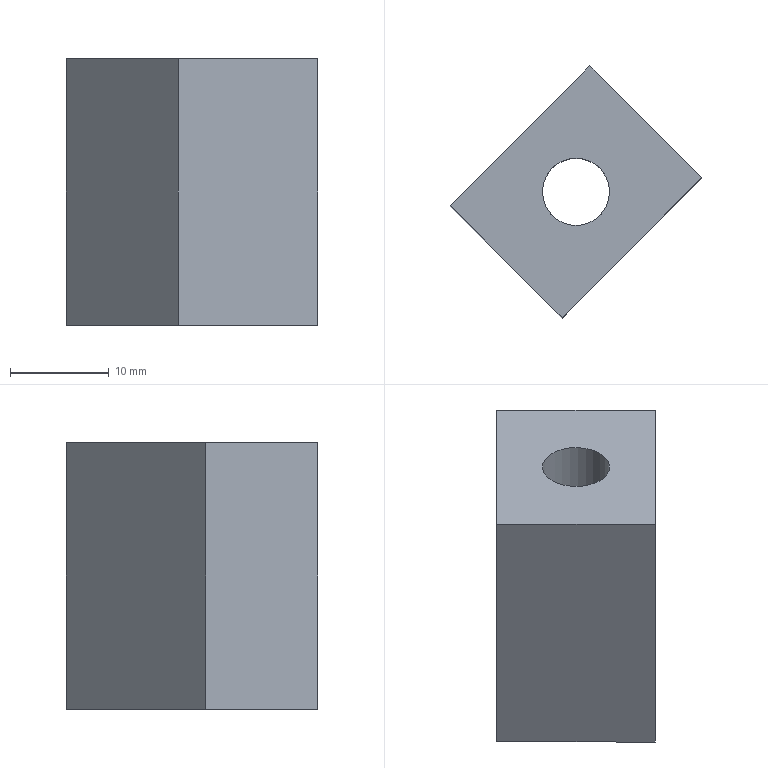Part | STEP file | gslz 2016.10.28-13_id1478_x_t | 1 solid | 9 faces | box 25.456 x 25.456 x 27 mm | volume 6738 mm3 | plane 7 | cylinder 2 | commonest cylinder face diameters 6.8 x1 12 x1
STEP:
#1=CARTESIAN_POINT('',(0.,0.,0.));
#2=DIRECTION('',(0.,0.,1.));
#3=DIRECTION('',(1.,0.,0.));
#4=AXIS2_PLACEMENT_3D('',#1,#2,#3);
#5=CARTESIAN_POINT('',(612.273,213.143,-70.5));
#6=VERTEX_POINT('',#5);
#7=CARTESIAN_POINT('',(608.873,213.143,-70.5));
#8=DIRECTION('',(0.,0.,-1.));
#9=DIRECTION('',(1.,0.,0.));
#10=AXIS2_PLACEMENT_3D('',#7,#8,#9);
#11=CIRCLE('',#10,3.4);
#12=CARTESIAN_POINT('',(628.559,232.788,-70.5));
#13=DIRECTION('',(0.,0.,1.));
#14=DIRECTION('',(1.,0.,0.));
#15=AXIS2_PLACEMENT_3D('',#12,#13,#14);
#16=PLANE('',#15);
#17=CARTESIAN_POINT('',(-16.286,-19.645));
#18=CARTESIAN_POINT('',(-16.286,-25.534));
#19=CARTESIAN_POINT('',(-21.386,-22.59));
#20=CARTESIAN_POINT('',(-26.486,-19.645));
#21=CARTESIAN_POINT('',(-21.386,-16.701));
#22=CARTESIAN_POINT('',(-16.286,-13.756));
#23=CARTESIAN_POINT('',(-16.286,-19.645));
#24=(BOUNDED_CURVE()B_SPLINE_CURVE(2,(#17,#18,#19,#20,#21,#22,#23),.UNSPECIFIED.,.T.,.F.)B_SPLINE_CURVE_WITH_KNOTS((1,2,2,2,2,1),(-2.094,0.,2.094,4.189,6.283,8.378),.UNSPECIFIED.)CURVE()GEOMETRIC_REPRESENTATION_ITEM()RATIONAL_B_SPLINE_CURVE((1.,0.5,1.,0.5,1.,0.5,1.))REPRESENTATION_ITEM(''));
#25=(GEOMETRIC_REPRESENTATION_CONTEXT(2)PARAMETRIC_REPRESENTATION_CONTEXT()REPRESENTATION_CONTEXT('',''));
#26=DEFINITIONAL_REPRESENTATION('',(#24),#25);
#27=PCURVE('',#16,#26);
#28=CARTESIAN_POINT('',(608.873,213.143,-55.5));
#29=DIRECTION('',(0.,0.,1.));
#30=DIRECTION('',(1.,0.,0.));
#31=AXIS2_PLACEMENT_3D('',#28,#29,#30);
#32=CYLINDRICAL_SURFACE('',#31,3.4);
#33=CARTESIAN_POINT('',(6.283,-15.));
#34=DIRECTION('',(-1.,0.));
#35=VECTOR('',#34,1.);
#36=LINE('',#33,#35);
#37=(GEOMETRIC_REPRESENTATION_CONTEXT(2)PARAMETRIC_REPRESENTATION_CONTEXT()REPRESENTATION_CONTEXT('',''));
#38=DEFINITIONAL_REPRESENTATION('',(#36),#37);
#39=PCURVE('',#32,#38);
#40=SURFACE_CURVE('',#11,(#27,#39),.PCURVE_S1.);
#41=EDGE_CURVE('',#6,#6,#40,.T.);
#42=ORIENTED_EDGE('',*,*,#41,.T.);
#43=EDGE_LOOP('',(#42));
#44=FACE_BOUND('',#43,.T.);
#45=CARTESIAN_POINT('',(621.601,214.557,-70.5));
#46=VERTEX_POINT('',#45);
#47=CARTESIAN_POINT('',(607.459,200.415,-70.5));
#48=VERTEX_POINT('',#47);
#49=CARTESIAN_POINT('',(623.015,215.971,-70.5));
#50=DIRECTION('',(-0.7071,-0.7071,0.));
#51=VECTOR('',#50,1.);
#52=LINE('',#49,#51);
#53=CARTESIAN_POINT('',(-5.544,-16.817));
#54=DIRECTION('',(-0.7071,-0.7071));
#55=VECTOR('',#54,1.);
#56=LINE('',#53,#55);
#57=(GEOMETRIC_REPRESENTATION_CONTEXT(2)PARAMETRIC_REPRESENTATION_CONTEXT()REPRESENTATION_CONTEXT('',''));
#58=DEFINITIONAL_REPRESENTATION('',(#56),#57);
#59=PCURVE('',#16,#58);
#60=CARTESIAN_POINT('',(623.015,215.971,-93.));
#61=DIRECTION('',(-0.7071,0.7071,0.));
#62=DIRECTION('',(-0.7071,-0.7071,0.));
#63=AXIS2_PLACEMENT_3D('',#60,#61,#62);
#64=PLANE('',#63);
#65=CARTESIAN_POINT('',(0.,22.5));
#66=DIRECTION('',(1.,0.));
#67=VECTOR('',#66,1.);
#68=LINE('',#65,#67);
#69=(GEOMETRIC_REPRESENTATION_CONTEXT(2)PARAMETRIC_REPRESENTATION_CONTEXT()REPRESENTATION_CONTEXT('',''));
#70=DEFINITIONAL_REPRESENTATION('',(#68),#69);
#71=PCURVE('',#64,#70);
#72=SURFACE_CURVE('',#52,(#59,#71),.PCURVE_S1.);
#73=EDGE_CURVE('',#46,#48,#72,.T.);
#74=ORIENTED_EDGE('',*,*,#73,.F.);
#75=CARTESIAN_POINT('',(610.287,225.87,-70.5));
#76=VERTEX_POINT('',#75);
#77=CARTESIAN_POINT('',(615.944,220.214,-70.5));
#78=DIRECTION('',(0.7071,-0.7071,0.));
#79=VECTOR('',#78,1.);
#80=LINE('',#77,#79);
#81=CARTESIAN_POINT('',(-12.615,-12.574));
#82=DIRECTION('',(0.7071,-0.7071));
#83=VECTOR('',#82,1.);
#84=LINE('',#81,#83);
#85=(GEOMETRIC_REPRESENTATION_CONTEXT(2)PARAMETRIC_REPRESENTATION_CONTEXT()REPRESENTATION_CONTEXT('',''));
#86=DEFINITIONAL_REPRESENTATION('',(#84),#85);
#87=PCURVE('',#16,#86);
#88=CARTESIAN_POINT('',(615.944,220.214,-93.));
#89=DIRECTION('',(-0.7071,-0.7071,0.));
#90=DIRECTION('',(0.7071,-0.7071,0.));
#91=AXIS2_PLACEMENT_3D('',#88,#89,#90);
#92=PLANE('',#91);
#93=CARTESIAN_POINT('',(0.,22.5));
#94=DIRECTION('',(1.,0.));
#95=VECTOR('',#94,1.);
#96=LINE('',#93,#95);
#97=(GEOMETRIC_REPRESENTATION_CONTEXT(2)PARAMETRIC_REPRESENTATION_CONTEXT()REPRESENTATION_CONTEXT('',''));
#98=DEFINITIONAL_REPRESENTATION('',(#96),#97);
#99=PCURVE('',#92,#98);
#100=SURFACE_CURVE('',#80,(#87,#99),.PCURVE_S1.);
#101=EDGE_CURVE('',#76,#46,#100,.T.);
#102=ORIENTED_EDGE('',*,*,#101,.F.);
#103=CARTESIAN_POINT('',(596.145,211.728,-70.5));
#104=VERTEX_POINT('',#103);
#105=CARTESIAN_POINT('',(611.701,227.285,-70.5));
#106=DIRECTION('',(-0.7071,-0.7071,0.));
#107=VECTOR('',#106,1.);
#108=LINE('',#105,#107);
#109=CARTESIAN_POINT('',(-16.858,-5.503));
#110=DIRECTION('',(-0.7071,-0.7071));
#111=VECTOR('',#110,1.);
#112=LINE('',#109,#111);
#113=(GEOMETRIC_REPRESENTATION_CONTEXT(2)PARAMETRIC_REPRESENTATION_CONTEXT()REPRESENTATION_CONTEXT('',''));
#114=DEFINITIONAL_REPRESENTATION('',(#112),#113);
#115=PCURVE('',#16,#114);
#116=CARTESIAN_POINT('',(611.701,227.285,-93.));
#117=DIRECTION('',(-0.7071,0.7071,0.));
#118=DIRECTION('',(-0.7071,-0.7071,0.));
#119=AXIS2_PLACEMENT_3D('',#116,#117,#118);
#120=PLANE('',#119);
#121=CARTESIAN_POINT('',(0.,22.5));
#122=DIRECTION('',(1.,0.));
#123=VECTOR('',#122,1.);
#124=LINE('',#121,#123);
#125=(GEOMETRIC_REPRESENTATION_CONTEXT(2)PARAMETRIC_REPRESENTATION_CONTEXT()REPRESENTATION_CONTEXT('',''));
#126=DEFINITIONAL_REPRESENTATION('',(#124),#125);
#127=PCURVE('',#120,#126);
#128=SURFACE_CURVE('',#108,(#115,#127),.PCURVE_S1.);
#129=EDGE_CURVE('',#76,#104,#128,.T.);
#130=ORIENTED_EDGE('',*,*,#129,.T.);
#131=CARTESIAN_POINT('',(601.822,206.051,-70.5));
#132=DIRECTION('',(0.7071,-0.7071,0.));
#133=VECTOR('',#132,1.);
#134=LINE('',#131,#133);
#135=CARTESIAN_POINT('',(-26.737,-26.737));
#136=DIRECTION('',(0.7071,-0.7071));
#137=VECTOR('',#136,1.);
#138=LINE('',#135,#137);
#139=(GEOMETRIC_REPRESENTATION_CONTEXT(2)PARAMETRIC_REPRESENTATION_CONTEXT()REPRESENTATION_CONTEXT('',''));
#140=DEFINITIONAL_REPRESENTATION('',(#138),#139);
#141=PCURVE('',#16,#140);
#142=CARTESIAN_POINT('',(601.822,206.051,-58.639));
#143=DIRECTION('',(0.7071,0.7071,0.));
#144=DIRECTION('',(-0.7071,0.7071,0.));
#145=AXIS2_PLACEMENT_3D('',#142,#143,#144);
#146=PLANE('',#145);
#147=CARTESIAN_POINT('',(0.,-11.861));
#148=DIRECTION('',(-1.,0.));
#149=VECTOR('',#148,1.);
#150=LINE('',#147,#149);
#151=(GEOMETRIC_REPRESENTATION_CONTEXT(2)PARAMETRIC_REPRESENTATION_CONTEXT()REPRESENTATION_CONTEXT('',''));
#152=DEFINITIONAL_REPRESENTATION('',(#150),#151);
#153=PCURVE('',#146,#152);
#154=SURFACE_CURVE('',#134,(#141,#153),.PCURVE_S1.);
#155=EDGE_CURVE('',#104,#48,#154,.T.);
#156=ORIENTED_EDGE('',*,*,#155,.T.);
#157=EDGE_LOOP('',(#74,#102,#130,#156));
#158=FACE_BOUND('',#157,.T.);
#159=ADVANCED_FACE('',(#44,#158),#16,.T.);
#160=CARTESIAN_POINT('',(621.601,214.557,-97.5));
#161=VERTEX_POINT('',#160);
#162=CARTESIAN_POINT('',(607.459,200.415,-97.5));
#163=VERTEX_POINT('',#162);
#164=CARTESIAN_POINT('',(623.015,215.971,-97.5));
#165=DIRECTION('',(-0.7071,-0.7071,0.));
#166=VECTOR('',#165,1.);
#167=LINE('',#164,#166);
#168=CARTESIAN_POINT('',(0.,-4.5));
#169=DIRECTION('',(1.,0.));
#170=VECTOR('',#169,1.);
#171=LINE('',#168,#170);
#172=(GEOMETRIC_REPRESENTATION_CONTEXT(2)PARAMETRIC_REPRESENTATION_CONTEXT()REPRESENTATION_CONTEXT('',''));
#173=DEFINITIONAL_REPRESENTATION('',(#171),#172);
#174=PCURVE('',#64,#173);
#175=CARTESIAN_POINT('',(617.358,221.628,-97.5));
#176=DIRECTION('',(0.,0.,1.));
#177=DIRECTION('',(1.,0.,0.));
#178=AXIS2_PLACEMENT_3D('',#175,#176,#177);
#179=PLANE('',#178);
#180=CARTESIAN_POINT('',(5.657,-5.657));
#181=DIRECTION('',(-0.7071,-0.7071));
#182=VECTOR('',#181,1.);
#183=LINE('',#180,#182);
#184=(GEOMETRIC_REPRESENTATION_CONTEXT(2)PARAMETRIC_REPRESENTATION_CONTEXT()REPRESENTATION_CONTEXT('',''));
#185=DEFINITIONAL_REPRESENTATION('',(#183),#184);
#186=PCURVE('',#179,#185);
#187=SURFACE_CURVE('',#167,(#174,#186),.PCURVE_S1.);
#188=EDGE_CURVE('',#161,#163,#187,.T.);
#189=ORIENTED_EDGE('',*,*,#188,.F.);
#190=CARTESIAN_POINT('',(621.601,214.557,-93.));
#191=DIRECTION('',(0.,0.,1.));
#192=VECTOR('',#191,1.);
#193=LINE('',#190,#192);
#194=CARTESIAN_POINT('',(2.,0.));
#195=DIRECTION('',(0.,1.));
#196=VECTOR('',#195,1.);
#197=LINE('',#194,#196);
#198=(GEOMETRIC_REPRESENTATION_CONTEXT(2)PARAMETRIC_REPRESENTATION_CONTEXT()REPRESENTATION_CONTEXT('',''));
#199=DEFINITIONAL_REPRESENTATION('',(#197),#198);
#200=PCURVE('',#64,#199);
#201=CARTESIAN_POINT('',(8.,0.));
#202=DIRECTION('',(0.,1.));
#203=VECTOR('',#202,1.);
#204=LINE('',#201,#203);
#205=(GEOMETRIC_REPRESENTATION_CONTEXT(2)PARAMETRIC_REPRESENTATION_CONTEXT()REPRESENTATION_CONTEXT('',''));
#206=DEFINITIONAL_REPRESENTATION('',(#204),#205);
#207=PCURVE('',#92,#206);
#208=SURFACE_CURVE('',#193,(#200,#207),.PCURVE_S1.);
#209=EDGE_CURVE('',#161,#46,#208,.T.);
#210=ORIENTED_EDGE('',*,*,#209,.T.);
#211=ORIENTED_EDGE('',*,*,#73,.T.);
#212=CARTESIAN_POINT('',(607.459,200.415,-93.));
#213=DIRECTION('',(0.,0.,1.));
#214=VECTOR('',#213,1.);
#215=LINE('',#212,#214);
#216=CARTESIAN_POINT('',(22.,0.));
#217=DIRECTION('',(0.,1.));
#218=VECTOR('',#217,1.);
#219=LINE('',#216,#218);
#220=(GEOMETRIC_REPRESENTATION_CONTEXT(2)PARAMETRIC_REPRESENTATION_CONTEXT()REPRESENTATION_CONTEXT('',''));
#221=DEFINITIONAL_REPRESENTATION('',(#219),#220);
#222=PCURVE('',#64,#221);
#223=CARTESIAN_POINT('',(-7.971,-34.361));
#224=DIRECTION('',(0.,1.));
#225=VECTOR('',#224,1.);
#226=LINE('',#223,#225);
#227=(GEOMETRIC_REPRESENTATION_CONTEXT(2)PARAMETRIC_REPRESENTATION_CONTEXT()REPRESENTATION_CONTEXT('',''));
#228=DEFINITIONAL_REPRESENTATION('',(#226),#227);
#229=PCURVE('',#146,#228);
#230=SURFACE_CURVE('',#215,(#222,#229),.PCURVE_S1.);
#231=EDGE_CURVE('',#163,#48,#230,.T.);
#232=ORIENTED_EDGE('',*,*,#231,.F.);
#233=EDGE_LOOP('',(#189,#210,#211,#232));
#234=FACE_BOUND('',#233,.T.);
#235=ADVANCED_FACE('',(#234),#64,.F.);
#236=CARTESIAN_POINT('',(614.873,213.143,-97.5));
#237=VERTEX_POINT('',#236);
#238=CARTESIAN_POINT('',(608.873,213.143,-97.5));
#239=DIRECTION('',(0.,0.,1.));
#240=DIRECTION('',(1.,0.,0.));
#241=AXIS2_PLACEMENT_3D('',#238,#239,#240);
#242=CIRCLE('',#241,6.);
#243=CARTESIAN_POINT('',(-8.485,-8.485));
#244=DIRECTION('',(1.,0.));
#245=AXIS2_PLACEMENT_2D('',#243,#244);
#246=CIRCLE('',#245,6.);
#247=(GEOMETRIC_REPRESENTATION_CONTEXT(2)PARAMETRIC_REPRESENTATION_CONTEXT()REPRESENTATION_CONTEXT('',''));
#248=DEFINITIONAL_REPRESENTATION('',(#246),#247);
#249=PCURVE('',#179,#248);
#250=CARTESIAN_POINT('',(608.873,213.143,-105.5));
#251=DIRECTION('',(0.,0.,1.));
#252=DIRECTION('',(1.,0.,0.));
#253=AXIS2_PLACEMENT_3D('',#250,#251,#252);
#254=CYLINDRICAL_SURFACE('',#253,6.);
#255=CARTESIAN_POINT('',(0.,8.));
#256=DIRECTION('',(1.,0.));
#257=VECTOR('',#256,1.);
#258=LINE('',#255,#257);
#259=(GEOMETRIC_REPRESENTATION_CONTEXT(2)PARAMETRIC_REPRESENTATION_CONTEXT()REPRESENTATION_CONTEXT('',''));
#260=DEFINITIONAL_REPRESENTATION('',(#258),#259);
#261=PCURVE('',#254,#260);
#262=SURFACE_CURVE('',#242,(#249,#261),.PCURVE_S1.);
#263=EDGE_CURVE('',#237,#237,#262,.T.);
#264=ORIENTED_EDGE('',*,*,#263,.T.);
#265=EDGE_LOOP('',(#264));
#266=FACE_BOUND('',#265,.T.);
#267=CARTESIAN_POINT('',(610.287,225.87,-97.5));
#268=VERTEX_POINT('',#267);
#269=CARTESIAN_POINT('',(615.944,220.214,-97.5));
#270=DIRECTION('',(-0.7071,0.7071,0.));
#271=VECTOR('',#270,1.);
#272=LINE('',#269,#271);
#273=CARTESIAN_POINT('',(-1.414,-1.414));
#274=DIRECTION('',(-0.7071,0.7071));
#275=VECTOR('',#274,1.);
#276=LINE('',#273,#275);
#277=(GEOMETRIC_REPRESENTATION_CONTEXT(2)PARAMETRIC_REPRESENTATION_CONTEXT()REPRESENTATION_CONTEXT('',''));
#278=DEFINITIONAL_REPRESENTATION('',(#276),#277);
#279=PCURVE('',#179,#278);
#280=CARTESIAN_POINT('',(0.,-4.5));
#281=DIRECTION('',(-1.,0.));
#282=VECTOR('',#281,1.);
#283=LINE('',#280,#282);
#284=(GEOMETRIC_REPRESENTATION_CONTEXT(2)PARAMETRIC_REPRESENTATION_CONTEXT()REPRESENTATION_CONTEXT('',''));
#285=DEFINITIONAL_REPRESENTATION('',(#283),#284);
#286=PCURVE('',#92,#285);
#287=SURFACE_CURVE('',#272,(#279,#286),.PCURVE_S1.);
#288=EDGE_CURVE('',#161,#268,#287,.T.);
#289=ORIENTED_EDGE('',*,*,#288,.F.);
#290=ORIENTED_EDGE('',*,*,#188,.T.);
#291=CARTESIAN_POINT('',(596.145,211.728,-97.5));
#292=VERTEX_POINT('',#291);
#293=CARTESIAN_POINT('',(601.822,206.051,-97.5));
#294=DIRECTION('',(-0.7071,0.7071,0.));
#295=VECTOR('',#294,1.);
#296=LINE('',#293,#295);
#297=CARTESIAN_POINT('',(-15.536,-15.577));
#298=DIRECTION('',(-0.7071,0.7071));
#299=VECTOR('',#298,1.);
#300=LINE('',#297,#299);
#301=(GEOMETRIC_REPRESENTATION_CONTEXT(2)PARAMETRIC_REPRESENTATION_CONTEXT()REPRESENTATION_CONTEXT('',''));
#302=DEFINITIONAL_REPRESENTATION('',(#300),#301);
#303=PCURVE('',#179,#302);
#304=CARTESIAN_POINT('',(0.,-38.861));
#305=DIRECTION('',(1.,0.));
#306=VECTOR('',#305,1.);
#307=LINE('',#304,#306);
#308=(GEOMETRIC_REPRESENTATION_CONTEXT(2)PARAMETRIC_REPRESENTATION_CONTEXT()REPRESENTATION_CONTEXT('',''));
#309=DEFINITIONAL_REPRESENTATION('',(#307),#308);
#310=PCURVE('',#146,#309);
#311=SURFACE_CURVE('',#296,(#303,#310),.PCURVE_S1.);
#312=EDGE_CURVE('',#163,#292,#311,.T.);
#313=ORIENTED_EDGE('',*,*,#312,.T.);
#314=CARTESIAN_POINT('',(611.701,227.285,-97.5));
#315=DIRECTION('',(-0.7071,-0.7071,0.));
#316=VECTOR('',#315,1.);
#317=LINE('',#314,#316);
#318=CARTESIAN_POINT('',(-5.657,5.657));
#319=DIRECTION('',(-0.7071,-0.7071));
#320=VECTOR('',#319,1.);
#321=LINE('',#318,#320);
#322=(GEOMETRIC_REPRESENTATION_CONTEXT(2)PARAMETRIC_REPRESENTATION_CONTEXT()REPRESENTATION_CONTEXT('',''));
#323=DEFINITIONAL_REPRESENTATION('',(#321),#322);
#324=PCURVE('',#179,#323);
#325=CARTESIAN_POINT('',(0.,-4.5));
#326=DIRECTION('',(1.,0.));
#327=VECTOR('',#326,1.);
#328=LINE('',#325,#327);
#329=(GEOMETRIC_REPRESENTATION_CONTEXT(2)PARAMETRIC_REPRESENTATION_CONTEXT()REPRESENTATION_CONTEXT('',''));
#330=DEFINITIONAL_REPRESENTATION('',(#328),#329);
#331=PCURVE('',#120,#330);
#332=SURFACE_CURVE('',#317,(#324,#331),.PCURVE_S1.);
#333=EDGE_CURVE('',#268,#292,#332,.T.);
#334=ORIENTED_EDGE('',*,*,#333,.F.);
#335=EDGE_LOOP('',(#289,#290,#313,#334));
#336=FACE_BOUND('',#335,.T.);
#337=ADVANCED_FACE('',(#266,#336),#179,.F.);
#338=ORIENTED_EDGE('',*,*,#129,.F.);
#339=CARTESIAN_POINT('',(610.287,225.87,-93.));
#340=DIRECTION('',(0.,0.,1.));
#341=VECTOR('',#340,1.);
#342=LINE('',#339,#341);
#343=CARTESIAN_POINT('',(2.,0.));
#344=DIRECTION('',(0.,1.));
#345=VECTOR('',#344,1.);
#346=LINE('',#343,#345);
#347=(GEOMETRIC_REPRESENTATION_CONTEXT(2)PARAMETRIC_REPRESENTATION_CONTEXT()REPRESENTATION_CONTEXT('',''));
#348=DEFINITIONAL_REPRESENTATION('',(#346),#347);
#349=PCURVE('',#120,#348);
#350=CARTESIAN_POINT('',(-8.,0.));
#351=DIRECTION('',(0.,1.));
#352=VECTOR('',#351,1.);
#353=LINE('',#350,#352);
#354=(GEOMETRIC_REPRESENTATION_CONTEXT(2)PARAMETRIC_REPRESENTATION_CONTEXT()REPRESENTATION_CONTEXT('',''));
#355=DEFINITIONAL_REPRESENTATION('',(#353),#354);
#356=PCURVE('',#92,#355);
#357=SURFACE_CURVE('',#342,(#349,#356),.PCURVE_S1.);
#358=EDGE_CURVE('',#268,#76,#357,.T.);
#359=ORIENTED_EDGE('',*,*,#358,.F.);
#360=ORIENTED_EDGE('',*,*,#333,.T.);
#361=CARTESIAN_POINT('',(596.145,211.728,-93.));
#362=DIRECTION('',(0.,0.,1.));
#363=VECTOR('',#362,1.);
#364=LINE('',#361,#363);
#365=CARTESIAN_POINT('',(22.,0.));
#366=DIRECTION('',(0.,1.));
#367=VECTOR('',#366,1.);
#368=LINE('',#365,#367);
#369=(GEOMETRIC_REPRESENTATION_CONTEXT(2)PARAMETRIC_REPRESENTATION_CONTEXT()REPRESENTATION_CONTEXT('',''));
#370=DEFINITIONAL_REPRESENTATION('',(#368),#369);
#371=PCURVE('',#120,#370);
#372=CARTESIAN_POINT('',(8.029,-34.361));
#373=DIRECTION('',(0.,1.));
#374=VECTOR('',#373,1.);
#375=LINE('',#372,#374);
#376=(GEOMETRIC_REPRESENTATION_CONTEXT(2)PARAMETRIC_REPRESENTATION_CONTEXT()REPRESENTATION_CONTEXT('',''));
#377=DEFINITIONAL_REPRESENTATION('',(#375),#376);
#378=PCURVE('',#146,#377);
#379=SURFACE_CURVE('',#364,(#371,#378),.PCURVE_S1.);
#380=EDGE_CURVE('',#292,#104,#379,.T.);
#381=ORIENTED_EDGE('',*,*,#380,.T.);
#382=EDGE_LOOP('',(#338,#359,#360,#381));
#383=FACE_BOUND('',#382,.T.);
#384=ADVANCED_FACE('',(#383),#120,.T.);
#385=ORIENTED_EDGE('',*,*,#101,.T.);
#386=ORIENTED_EDGE('',*,*,#209,.F.);
#387=ORIENTED_EDGE('',*,*,#288,.T.);
#388=ORIENTED_EDGE('',*,*,#358,.T.);
#389=EDGE_LOOP('',(#385,#386,#387,#388));
#390=FACE_BOUND('',#389,.T.);
#391=ADVANCED_FACE('',(#390),#92,.F.);
#392=ORIENTED_EDGE('',*,*,#155,.F.);
#393=ORIENTED_EDGE('',*,*,#380,.F.);
#394=ORIENTED_EDGE('',*,*,#312,.F.);
#395=ORIENTED_EDGE('',*,*,#231,.T.);
#396=EDGE_LOOP('',(#392,#393,#394,#395));
#397=FACE_BOUND('',#396,.T.);
#398=ADVANCED_FACE('',(#397),#146,.F.);
#399=CARTESIAN_POINT('',(612.273,213.143,-85.5));
#400=VERTEX_POINT('',#399);
#401=CARTESIAN_POINT('',(608.873,213.143,-85.5));
#402=DIRECTION('',(0.,0.,-1.));
#403=DIRECTION('',(1.,0.,0.));
#404=AXIS2_PLACEMENT_3D('',#401,#402,#403);
#405=CIRCLE('',#404,3.4);
#406=CARTESIAN_POINT('',(6.283,-30.));
#407=DIRECTION('',(-1.,0.));
#408=VECTOR('',#407,1.);
#409=LINE('',#406,#408);
#410=(GEOMETRIC_REPRESENTATION_CONTEXT(2)PARAMETRIC_REPRESENTATION_CONTEXT()REPRESENTATION_CONTEXT('',''));
#411=DEFINITIONAL_REPRESENTATION('',(#409),#410);
#412=PCURVE('',#32,#411);
#413=CARTESIAN_POINT('',(608.873,213.143,-85.5));
#414=DIRECTION('',(0.,0.,1.));
#415=DIRECTION('',(1.,0.,0.));
#416=AXIS2_PLACEMENT_3D('',#413,#414,#415);
#417=PLANE('',#416);
#418=CARTESIAN_POINT('',(3.4,0.));
#419=CARTESIAN_POINT('',(3.4,-5.889));
#420=CARTESIAN_POINT('',(-1.7,-2.944));
#421=CARTESIAN_POINT('',(-6.8,0.));
#422=CARTESIAN_POINT('',(-1.7,2.944));
#423=CARTESIAN_POINT('',(3.4,5.889));
#424=CARTESIAN_POINT('',(3.4,0.));
#425=(BOUNDED_CURVE()B_SPLINE_CURVE(2,(#418,#419,#420,#421,#422,#423,#424),.UNSPECIFIED.,.T.,.F.)B_SPLINE_CURVE_WITH_KNOTS((1,2,2,2,2,1),(-2.094,0.,2.094,4.189,6.283,8.378),.UNSPECIFIED.)CURVE()GEOMETRIC_REPRESENTATION_ITEM()RATIONAL_B_SPLINE_CURVE((1.,0.5,1.,0.5,1.,0.5,1.))REPRESENTATION_ITEM(''));
#426=(GEOMETRIC_REPRESENTATION_CONTEXT(2)PARAMETRIC_REPRESENTATION_CONTEXT()REPRESENTATION_CONTEXT('',''));
#427=DEFINITIONAL_REPRESENTATION('',(#425),#426);
#428=PCURVE('',#417,#427);
#429=SURFACE_CURVE('',#405,(#412,#428),.PCURVE_S1.);
#430=EDGE_CURVE('',#400,#400,#429,.T.);
#431=ORIENTED_EDGE('',*,*,#430,.F.);
#432=CARTESIAN_POINT('',(612.273,213.143,-85.5));
#433=CARTESIAN_POINT('',(612.273,213.143,-70.5));
#434=B_SPLINE_CURVE_WITH_KNOTS('',1,(#432,#433),.UNSPECIFIED.,.F.,.F.,(2,2),(-30.,-15.),.PIECEWISE_BEZIER_KNOTS.);
#435=CARTESIAN_POINT('',(6.283,0.));
#436=DIRECTION('',(0.,1.));
#437=VECTOR('',#436,1.);
#438=LINE('',#435,#437);
#439=(GEOMETRIC_REPRESENTATION_CONTEXT(2)PARAMETRIC_REPRESENTATION_CONTEXT()REPRESENTATION_CONTEXT('',''));
#440=DEFINITIONAL_REPRESENTATION('',(#438),#439);
#441=PCURVE('',#32,#440);
#442=CARTESIAN_POINT('',(0.,0.));
#443=DIRECTION('',(0.,1.));
#444=VECTOR('',#443,1.);
#445=LINE('',#442,#444);
#446=(GEOMETRIC_REPRESENTATION_CONTEXT(2)PARAMETRIC_REPRESENTATION_CONTEXT()REPRESENTATION_CONTEXT('',''));
#447=DEFINITIONAL_REPRESENTATION('',(#445),#446);
#448=PCURVE('',#32,#447);
#449=SEAM_CURVE('',#434,(#441,#448),.PCURVE_S1.);
#450=EDGE_CURVE('',#400,#6,#449,.T.);
#451=ORIENTED_EDGE('',*,*,#450,.T.);
#452=ORIENTED_EDGE('',*,*,#41,.T.);
#453=ORIENTED_EDGE('',*,*,#450,.F.);
#454=EDGE_LOOP('',(#431,#451,#452,#453));
#455=FACE_BOUND('',#454,.F.);
#456=ADVANCED_FACE('',(#455),#32,.F.);
#457=ORIENTED_EDGE('',*,*,#430,.F.);
#458=EDGE_LOOP('',(#457));
#459=FACE_BOUND('',#458,.T.);
#460=CARTESIAN_POINT('',(614.873,213.143,-85.5));
#461=VERTEX_POINT('',#460);
#462=CARTESIAN_POINT('',(608.873,213.143,-85.5));
#463=DIRECTION('',(0.,0.,-1.));
#464=DIRECTION('',(1.,0.,0.));
#465=AXIS2_PLACEMENT_3D('',#462,#463,#464);
#466=CIRCLE('',#465,6.);
#467=CARTESIAN_POINT('',(6.,0.));
#468=CARTESIAN_POINT('',(6.,-10.392));
#469=CARTESIAN_POINT('',(-3.,-5.196));
#470=CARTESIAN_POINT('',(-12.,0.));
#471=CARTESIAN_POINT('',(-3.,5.196));
#472=CARTESIAN_POINT('',(6.,10.392));
#473=CARTESIAN_POINT('',(6.,0.));
#474=(BOUNDED_CURVE()B_SPLINE_CURVE(2,(#467,#468,#469,#470,#471,#472,#473),.UNSPECIFIED.,.T.,.F.)B_SPLINE_CURVE_WITH_KNOTS((1,2,2,2,2,1),(-2.094,0.,2.094,4.189,6.283,8.378),.UNSPECIFIED.)CURVE()GEOMETRIC_REPRESENTATION_ITEM()RATIONAL_B_SPLINE_CURVE((1.,0.5,1.,0.5,1.,0.5,1.))REPRESENTATION_ITEM(''));
#475=(GEOMETRIC_REPRESENTATION_CONTEXT(2)PARAMETRIC_REPRESENTATION_CONTEXT()REPRESENTATION_CONTEXT('',''));
#476=DEFINITIONAL_REPRESENTATION('',(#474),#475);
#477=PCURVE('',#417,#476);
#478=CARTESIAN_POINT('',(6.283,20.));
#479=DIRECTION('',(-1.,0.));
#480=VECTOR('',#479,1.);
#481=LINE('',#478,#480);
#482=(GEOMETRIC_REPRESENTATION_CONTEXT(2)PARAMETRIC_REPRESENTATION_CONTEXT()REPRESENTATION_CONTEXT('',''));
#483=DEFINITIONAL_REPRESENTATION('',(#481),#482);
#484=PCURVE('',#254,#483);
#485=SURFACE_CURVE('',#466,(#477,#484),.PCURVE_S1.);
#486=EDGE_CURVE('',#461,#461,#485,.T.);
#487=ORIENTED_EDGE('',*,*,#486,.T.);
#488=EDGE_LOOP('',(#487));
#489=FACE_BOUND('',#488,.T.);
#490=ADVANCED_FACE('',(#459,#489),#417,.F.);
#491=ORIENTED_EDGE('',*,*,#486,.T.);
#492=CARTESIAN_POINT('',(614.873,213.143,-97.5));
#493=CARTESIAN_POINT('',(614.873,213.143,-85.5));
#494=B_SPLINE_CURVE_WITH_KNOTS('',1,(#492,#493),.UNSPECIFIED.,.F.,.F.,(2,2),(8.,20.),.PIECEWISE_BEZIER_KNOTS.);
#495=CARTESIAN_POINT('',(0.,0.));
#496=DIRECTION('',(0.,1.));
#497=VECTOR('',#496,1.);
#498=LINE('',#495,#497);
#499=(GEOMETRIC_REPRESENTATION_CONTEXT(2)PARAMETRIC_REPRESENTATION_CONTEXT()REPRESENTATION_CONTEXT('',''));
#500=DEFINITIONAL_REPRESENTATION('',(#498),#499);
#501=PCURVE('',#254,#500);
#502=CARTESIAN_POINT('',(6.283,0.));
#503=DIRECTION('',(0.,1.));
#504=VECTOR('',#503,1.);
#505=LINE('',#502,#504);
#506=(GEOMETRIC_REPRESENTATION_CONTEXT(2)PARAMETRIC_REPRESENTATION_CONTEXT()REPRESENTATION_CONTEXT('',''));
#507=DEFINITIONAL_REPRESENTATION('',(#505),#506);
#508=PCURVE('',#254,#507);
#509=SEAM_CURVE('',#494,(#501,#508),.PCURVE_S1.);
#510=EDGE_CURVE('',#237,#461,#509,.T.);
#511=ORIENTED_EDGE('',*,*,#510,.F.);
#512=ORIENTED_EDGE('',*,*,#263,.T.);
#513=ORIENTED_EDGE('',*,*,#510,.T.);
#514=EDGE_LOOP('',(#491,#511,#512,#513));
#515=FACE_BOUND('',#514,.F.);
#516=ADVANCED_FACE('',(#515),#254,.F.);
#517=CLOSED_SHELL('',(#159,#235,#337,#384,#391,#398,#456,#490,#516));
#518=MANIFOLD_SOLID_BREP('',#517);
#519=(LENGTH_UNIT()NAMED_UNIT(*)SI_UNIT(.MILLI.,.METRE.));
#520=UNCERTAINTY_MEASURE_WITH_UNIT(LENGTH_MEASURE(0.000002),#519,'','');
#521=(NAMED_UNIT(*)PLANE_ANGLE_UNIT()SI_UNIT($,.RADIAN.));
#522=(NAMED_UNIT(*)SI_UNIT($,.STERADIAN.)SOLID_ANGLE_UNIT());
#523=(GEOMETRIC_REPRESENTATION_CONTEXT(3)GLOBAL_UNCERTAINTY_ASSIGNED_CONTEXT((#520))GLOBAL_UNIT_ASSIGNED_CONTEXT((#519,#521,#522))REPRESENTATION_CONTEXT('',''));
#524=ADVANCED_BREP_SHAPE_REPRESENTATION('',(#4,#518),#523);